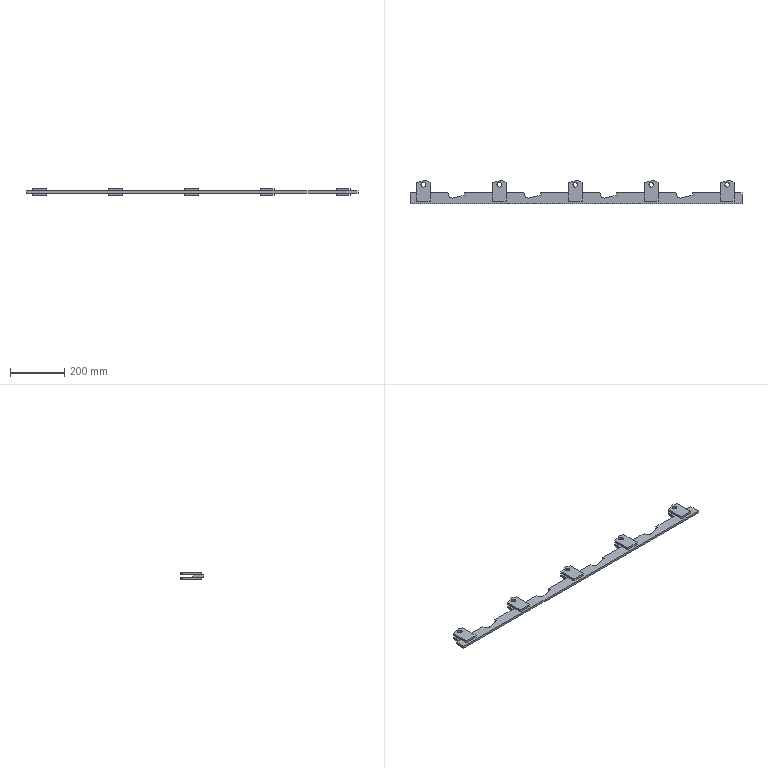Part | STEP file | Connecting plate assembly 2_Default<As machined> | 11 solids | 116 faces | box 1223 x 86.845 x 24 mm | volume 635186 mm3 | plane 92 | cylinder 24 | commonest cylinder face diameters 17 x20 30 x4